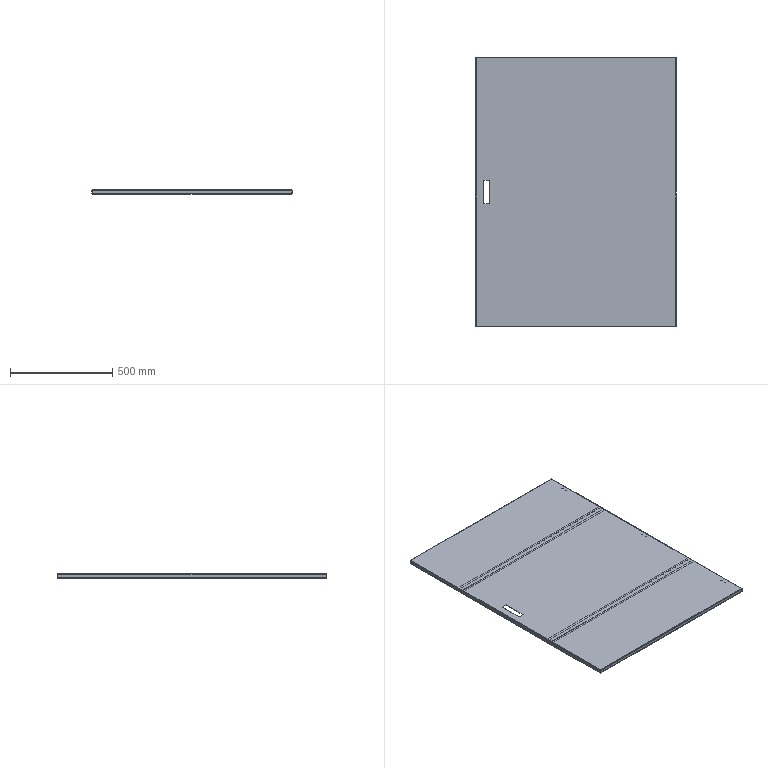Part | NX | features BREP 3 | 3 solids | 192 faces | box 982 x 1320 x 20 mm | volume 3020996 mm3 | plane 126 | cylinder 50 | spline 16 | commonest cylinder face diameters 6 x12 4 x11 8 x11 1.473 x8 4.473 x8